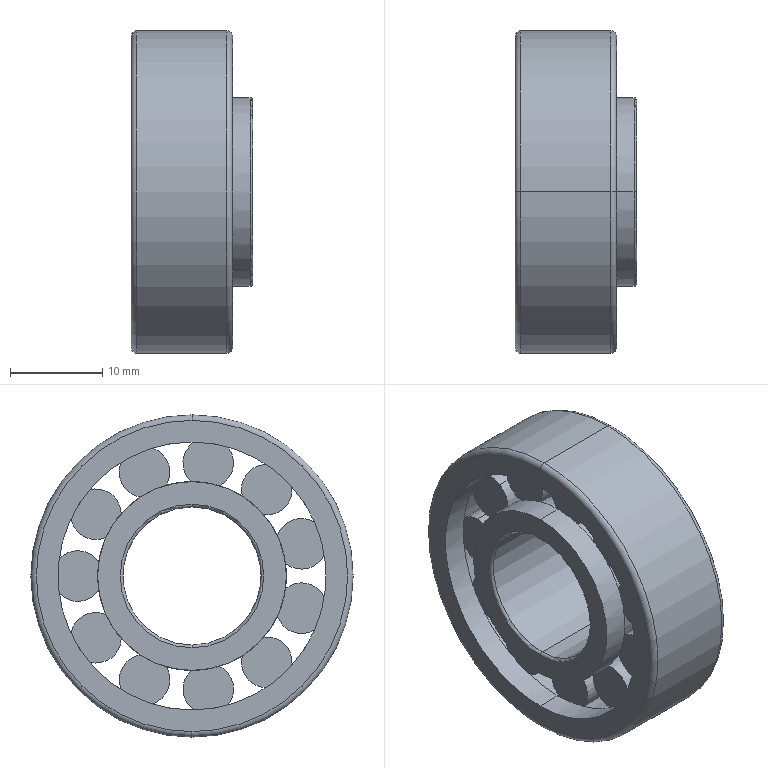Part | SolidWorks | features Revolution 4, CirPattern 1 | 1 solid | 154 faces | box 13.2 x 35 x 35 mm | volume 6194 mm3 | cylinder 71 | plane 71 | torus 12 | commonest cylinder face diameters 5.5 x33 19.3 x12 30.3 x12 15 x4 20.5 x4 29.1 x4